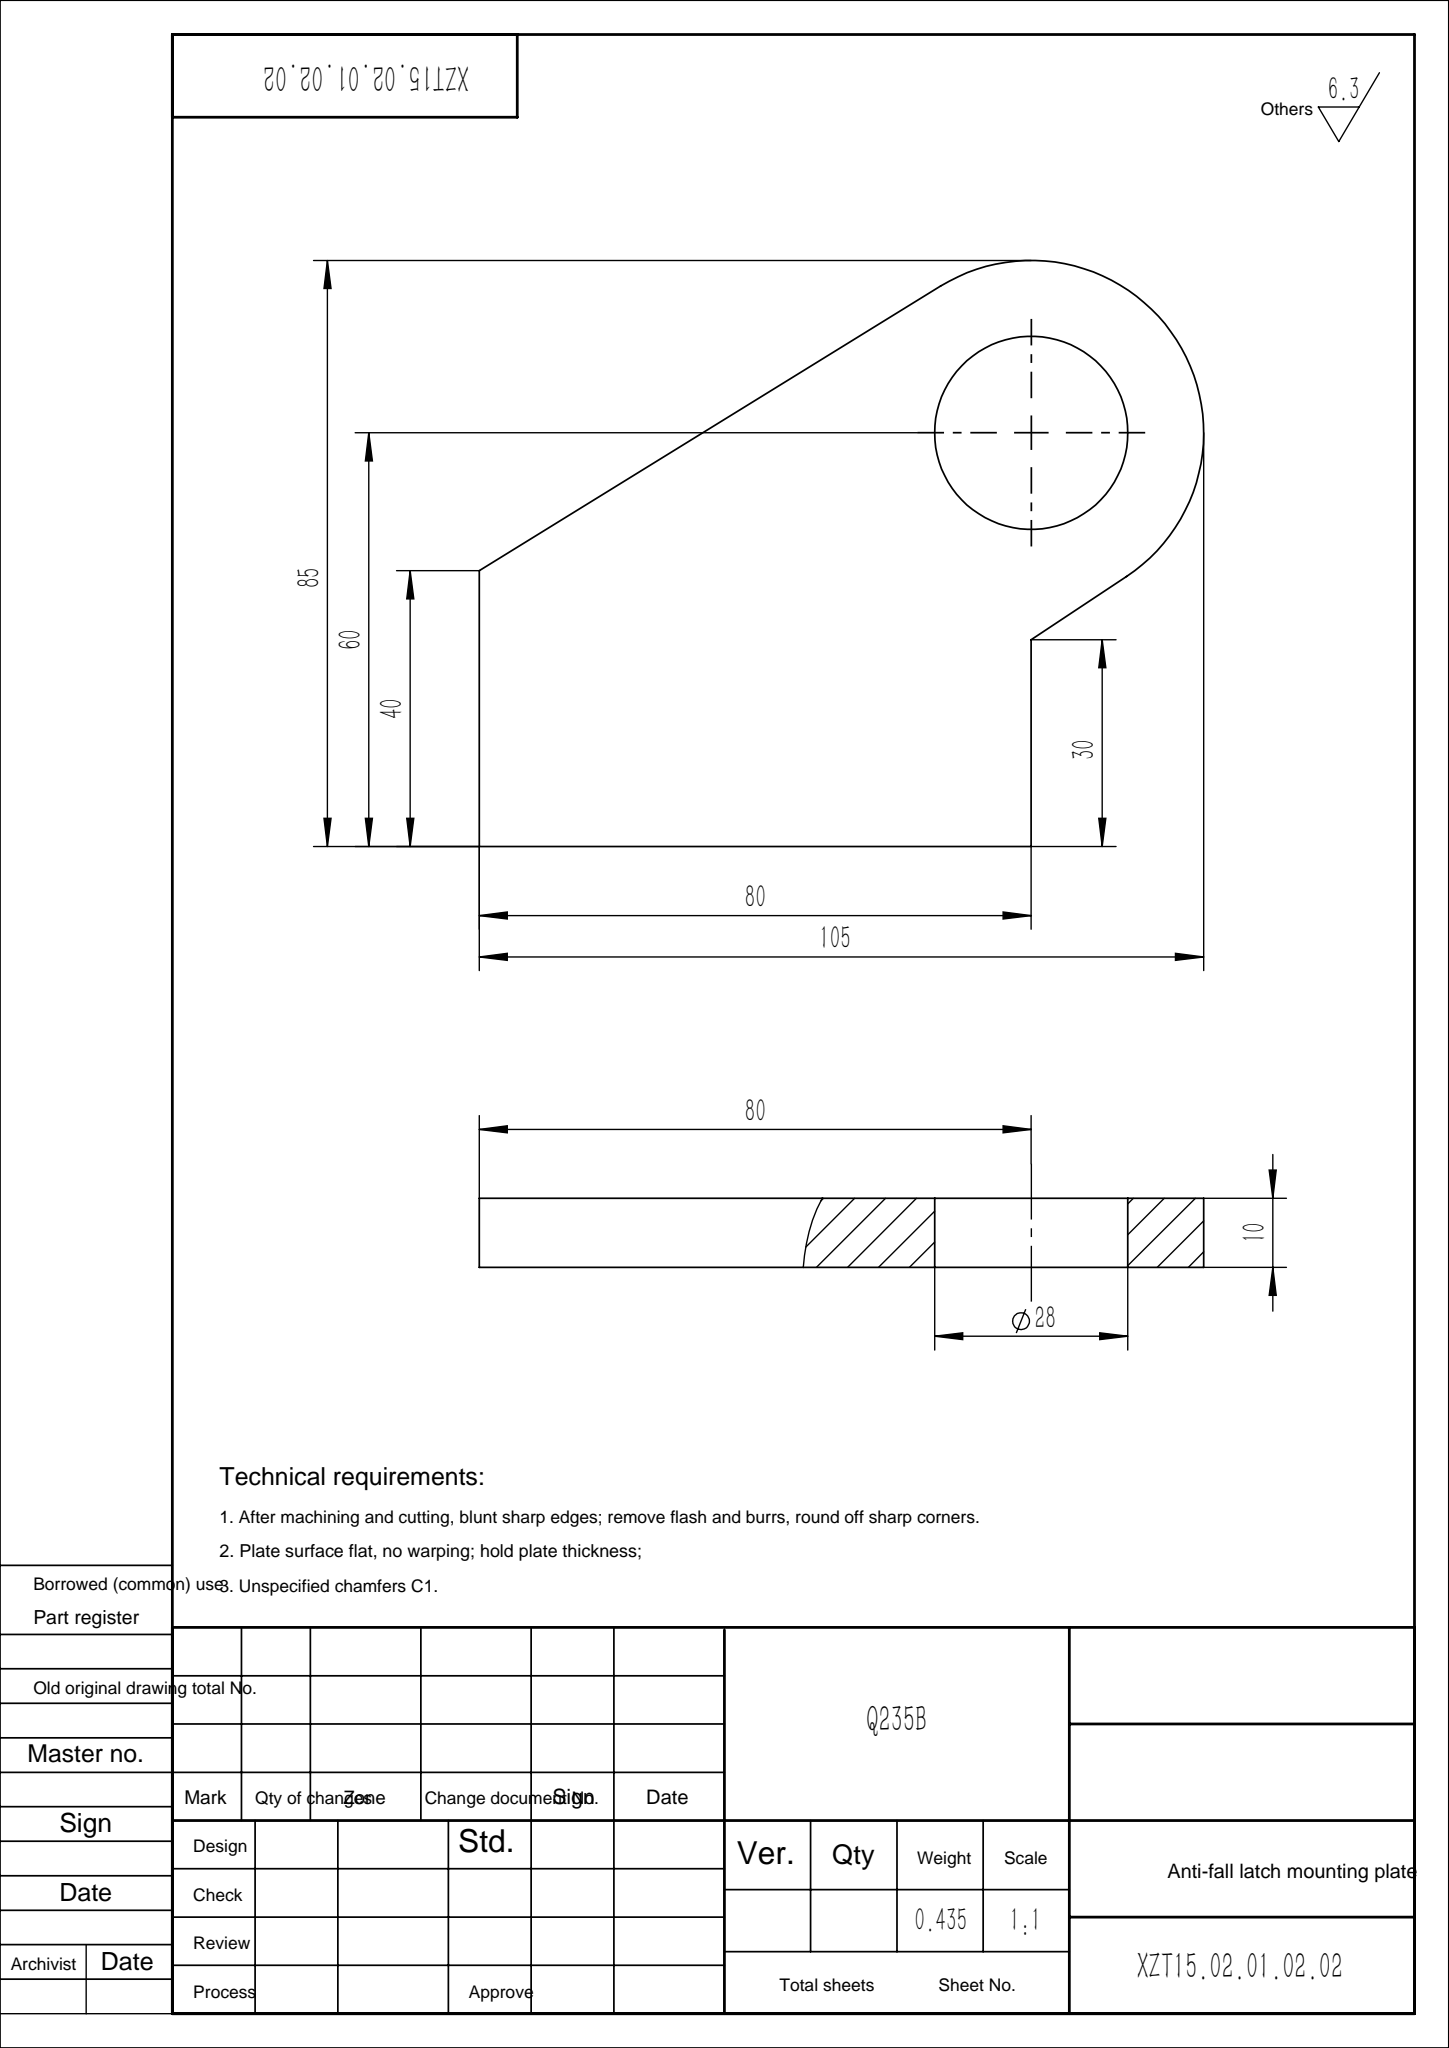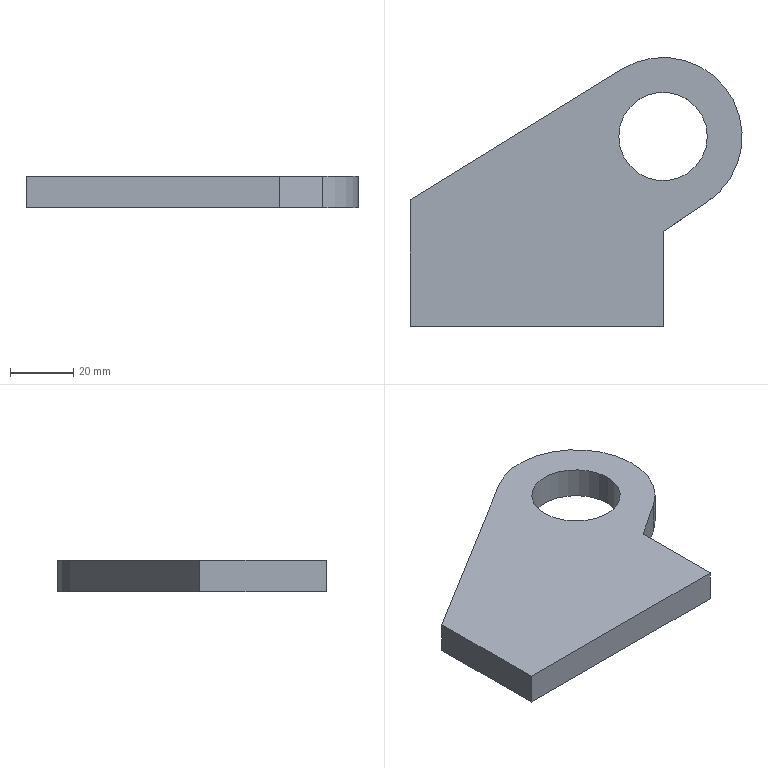Part | SolidWorks | features Extrusion 1 | 1 solid | 10 faces | box 105 x 85 x 10 mm | volume 55453 mm3 | plane 7 | cylinder 3 | commonest cylinder face diameters 28 x2 50 x1
STEP:
#1=CARTESIAN_POINT('',(66.,60.,5.));
#2=VERTEX_POINT('',#1);
#3=CARTESIAN_POINT('',(94.,60.,5.));
#4=VERTEX_POINT('',#3);
#5=CARTESIAN_POINT('',(80.,60.,5.));
#6=DIRECTION('',(0.,0.,1.));
#7=DIRECTION('',(1.,0.,0.));
#8=AXIS2_PLACEMENT_3D('',#5,#6,#7);
#9=CIRCLE('',#8,14.);
#10=EDGE_CURVE('',#2,#4,#9,.T.);
#11=ORIENTED_EDGE('',*,*,#10,.T.);
#12=CARTESIAN_POINT('',(94.,60.,-5.));
#13=VERTEX_POINT('',#12);
#14=CARTESIAN_POINT('',(94.,60.,5.));
#15=DIRECTION('',(0.,0.,-1.));
#16=VECTOR('',#15,1000.);
#17=LINE('',#14,#16);
#18=EDGE_CURVE('',#4,#13,#17,.T.);
#19=ORIENTED_EDGE('',*,*,#18,.T.);
#20=CARTESIAN_POINT('',(66.,60.,-5.));
#21=VERTEX_POINT('',#20);
#22=CARTESIAN_POINT('',(80.,60.,-5.));
#23=DIRECTION('',(0.,0.,1.));
#24=DIRECTION('',(1.,0.,0.));
#25=AXIS2_PLACEMENT_3D('',#22,#23,#24);
#26=CIRCLE('',#25,14.);
#27=EDGE_CURVE('',#21,#13,#26,.T.);
#28=ORIENTED_EDGE('',*,*,#27,.F.);
#29=CARTESIAN_POINT('',(66.,60.,5.));
#30=DIRECTION('',(0.,0.,-1.));
#31=VECTOR('',#30,1000.);
#32=LINE('',#29,#31);
#33=EDGE_CURVE('',#2,#21,#32,.T.);
#34=ORIENTED_EDGE('',*,*,#33,.F.);
#35=EDGE_LOOP('',(#11,#19,#28,#34));
#36=FACE_OUTER_BOUND('',#35,.T.);
#37=CARTESIAN_POINT('',(80.,60.,5.));
#38=DIRECTION('',(0.,0.,-1.));
#39=DIRECTION('',(-1.,0.,0.));
#40=AXIS2_PLACEMENT_3D('',#37,#38,#39);
#41=CYLINDRICAL_SURFACE('',#40,14.);
#42=ADVANCED_FACE('',(#36),#41,.F.);
#43=CARTESIAN_POINT('',(0.,0.,5.));
#44=VERTEX_POINT('',#43);
#45=CARTESIAN_POINT('',(80.,0.,5.));
#46=VERTEX_POINT('',#45);
#47=CARTESIAN_POINT('',(80.,0.,5.));
#48=DIRECTION('',(1.,0.,0.));
#49=VECTOR('',#48,1000.);
#50=LINE('',#47,#49);
#51=EDGE_CURVE('',#44,#46,#50,.T.);
#52=ORIENTED_EDGE('',*,*,#51,.T.);
#53=CARTESIAN_POINT('',(80.,30.,5.));
#54=VERTEX_POINT('',#53);
#55=CARTESIAN_POINT('',(80.,30.,5.));
#56=DIRECTION('',(0.,1.,0.));
#57=VECTOR('',#56,1000.);
#58=LINE('',#55,#57);
#59=EDGE_CURVE('',#46,#54,#58,.T.);
#60=ORIENTED_EDGE('',*,*,#59,.T.);
#61=CARTESIAN_POINT('',(93.819,39.167,5.));
#62=VERTEX_POINT('',#61);
#63=CARTESIAN_POINT('',(80.,30.,5.));
#64=DIRECTION('',(0.8333,0.5528,0.));
#65=VECTOR('',#64,1000.);
#66=LINE('',#63,#65);
#67=EDGE_CURVE('',#54,#62,#66,.T.);
#68=ORIENTED_EDGE('',*,*,#67,.T.);
#69=CARTESIAN_POINT('',(66.869,81.274,5.));
#70=VERTEX_POINT('',#69);
#71=CARTESIAN_POINT('',(80.,60.,5.));
#72=DIRECTION('',(0.,0.,1.));
#73=DIRECTION('',(-1.,0.,0.));
#74=AXIS2_PLACEMENT_3D('',#71,#72,#73);
#75=CIRCLE('',#74,25.);
#76=EDGE_CURVE('',#62,#70,#75,.T.);
#77=ORIENTED_EDGE('',*,*,#76,.T.);
#78=CARTESIAN_POINT('',(0.,40.,5.));
#79=VERTEX_POINT('',#78);
#80=CARTESIAN_POINT('',(0.,40.,5.));
#81=DIRECTION('',(-0.851,-0.5252,0.));
#82=VECTOR('',#81,1000.);
#83=LINE('',#80,#82);
#84=EDGE_CURVE('',#70,#79,#83,.T.);
#85=ORIENTED_EDGE('',*,*,#84,.T.);
#86=CARTESIAN_POINT('',(0.,0.,5.));
#87=DIRECTION('',(0.,-1.,0.));
#88=VECTOR('',#87,1000.);
#89=LINE('',#86,#88);
#90=EDGE_CURVE('',#79,#44,#89,.T.);
#91=ORIENTED_EDGE('',*,*,#90,.T.);
#92=EDGE_LOOP('',(#52,#60,#68,#77,#85,#91));
#93=FACE_OUTER_BOUND('',#92,.T.);
#94=ORIENTED_EDGE('',*,*,#10,.F.);
#95=CARTESIAN_POINT('',(80.,60.,5.));
#96=DIRECTION('',(0.,0.,1.));
#97=DIRECTION('',(1.,0.,0.));
#98=AXIS2_PLACEMENT_3D('',#95,#96,#97);
#99=CIRCLE('',#98,14.);
#100=EDGE_CURVE('',#4,#2,#99,.T.);
#101=ORIENTED_EDGE('',*,*,#100,.F.);
#102=EDGE_LOOP('',(#94,#101));
#103=FACE_BOUND('',#102,.T.);
#104=CARTESIAN_POINT('',(80.,60.,5.));
#105=DIRECTION('',(0.,0.,-1.));
#106=DIRECTION('',(-1.,0.,0.));
#107=AXIS2_PLACEMENT_3D('',#104,#105,#106);
#108=PLANE('',#107);
#109=ADVANCED_FACE('',(#93,#103),#108,.F.);
#110=CARTESIAN_POINT('',(0.,0.,-5.));
#111=VERTEX_POINT('',#110);
#112=CARTESIAN_POINT('',(80.,0.,-5.));
#113=VERTEX_POINT('',#112);
#114=CARTESIAN_POINT('',(80.,0.,-5.));
#115=DIRECTION('',(1.,0.,0.));
#116=VECTOR('',#115,1000.);
#117=LINE('',#114,#116);
#118=EDGE_CURVE('',#111,#113,#117,.T.);
#119=ORIENTED_EDGE('',*,*,#118,.F.);
#120=CARTESIAN_POINT('',(0.,40.,-5.));
#121=VERTEX_POINT('',#120);
#122=CARTESIAN_POINT('',(0.,0.,-5.));
#123=DIRECTION('',(0.,-1.,0.));
#124=VECTOR('',#123,1000.);
#125=LINE('',#122,#124);
#126=EDGE_CURVE('',#121,#111,#125,.T.);
#127=ORIENTED_EDGE('',*,*,#126,.F.);
#128=CARTESIAN_POINT('',(66.869,81.274,-5.));
#129=VERTEX_POINT('',#128);
#130=CARTESIAN_POINT('',(0.,40.,-5.));
#131=DIRECTION('',(-0.851,-0.5252,0.));
#132=VECTOR('',#131,1000.);
#133=LINE('',#130,#132);
#134=EDGE_CURVE('',#129,#121,#133,.T.);
#135=ORIENTED_EDGE('',*,*,#134,.F.);
#136=CARTESIAN_POINT('',(93.819,39.167,-5.));
#137=VERTEX_POINT('',#136);
#138=CARTESIAN_POINT('',(80.,60.,-5.));
#139=DIRECTION('',(0.,0.,1.));
#140=DIRECTION('',(-1.,0.,0.));
#141=AXIS2_PLACEMENT_3D('',#138,#139,#140);
#142=CIRCLE('',#141,25.);
#143=EDGE_CURVE('',#137,#129,#142,.T.);
#144=ORIENTED_EDGE('',*,*,#143,.F.);
#145=CARTESIAN_POINT('',(80.,30.,-5.));
#146=VERTEX_POINT('',#145);
#147=CARTESIAN_POINT('',(80.,30.,-5.));
#148=DIRECTION('',(0.8333,0.5528,0.));
#149=VECTOR('',#148,1000.);
#150=LINE('',#147,#149);
#151=EDGE_CURVE('',#146,#137,#150,.T.);
#152=ORIENTED_EDGE('',*,*,#151,.F.);
#153=CARTESIAN_POINT('',(80.,30.,-5.));
#154=DIRECTION('',(0.,1.,0.));
#155=VECTOR('',#154,1000.);
#156=LINE('',#153,#155);
#157=EDGE_CURVE('',#113,#146,#156,.T.);
#158=ORIENTED_EDGE('',*,*,#157,.F.);
#159=EDGE_LOOP('',(#119,#127,#135,#144,#152,#158));
#160=FACE_OUTER_BOUND('',#159,.T.);
#161=ORIENTED_EDGE('',*,*,#27,.T.);
#162=CARTESIAN_POINT('',(80.,60.,-5.));
#163=DIRECTION('',(0.,0.,1.));
#164=DIRECTION('',(1.,0.,0.));
#165=AXIS2_PLACEMENT_3D('',#162,#163,#164);
#166=CIRCLE('',#165,14.);
#167=EDGE_CURVE('',#13,#21,#166,.T.);
#168=ORIENTED_EDGE('',*,*,#167,.T.);
#169=EDGE_LOOP('',(#161,#168));
#170=FACE_BOUND('',#169,.T.);
#171=CARTESIAN_POINT('',(80.,60.,-5.));
#172=DIRECTION('',(0.,0.,-1.));
#173=DIRECTION('',(-1.,0.,0.));
#174=AXIS2_PLACEMENT_3D('',#171,#172,#173);
#175=PLANE('',#174);
#176=ADVANCED_FACE('',(#160,#170),#175,.T.);
#177=ORIENTED_EDGE('',*,*,#118,.T.);
#178=CARTESIAN_POINT('',(80.,0.,5.));
#179=DIRECTION('',(0.,0.,-1.));
#180=VECTOR('',#179,1000.);
#181=LINE('',#178,#180);
#182=EDGE_CURVE('',#46,#113,#181,.T.);
#183=ORIENTED_EDGE('',*,*,#182,.F.);
#184=ORIENTED_EDGE('',*,*,#51,.F.);
#185=CARTESIAN_POINT('',(0.,0.,5.));
#186=DIRECTION('',(0.,0.,-1.));
#187=VECTOR('',#186,1000.);
#188=LINE('',#185,#187);
#189=EDGE_CURVE('',#44,#111,#188,.T.);
#190=ORIENTED_EDGE('',*,*,#189,.T.);
#191=EDGE_LOOP('',(#177,#183,#184,#190));
#192=FACE_OUTER_BOUND('',#191,.T.);
#193=CARTESIAN_POINT('',(80.,0.,5.));
#194=DIRECTION('',(0.,1.,0.));
#195=DIRECTION('',(0.,0.,1.));
#196=AXIS2_PLACEMENT_3D('',#193,#194,#195);
#197=PLANE('',#196);
#198=ADVANCED_FACE('',(#192),#197,.F.);
#199=ORIENTED_EDGE('',*,*,#157,.T.);
#200=CARTESIAN_POINT('',(80.,30.,5.));
#201=DIRECTION('',(0.,0.,-1.));
#202=VECTOR('',#201,1000.);
#203=LINE('',#200,#202);
#204=EDGE_CURVE('',#54,#146,#203,.T.);
#205=ORIENTED_EDGE('',*,*,#204,.F.);
#206=ORIENTED_EDGE('',*,*,#59,.F.);
#207=ORIENTED_EDGE('',*,*,#182,.T.);
#208=EDGE_LOOP('',(#199,#205,#206,#207));
#209=FACE_OUTER_BOUND('',#208,.T.);
#210=CARTESIAN_POINT('',(80.,30.,5.));
#211=DIRECTION('',(-1.,0.,0.));
#212=DIRECTION('',(0.,0.,1.));
#213=AXIS2_PLACEMENT_3D('',#210,#211,#212);
#214=PLANE('',#213);
#215=ADVANCED_FACE('',(#209),#214,.F.);
#216=ORIENTED_EDGE('',*,*,#151,.T.);
#217=CARTESIAN_POINT('',(93.819,39.167,5.));
#218=DIRECTION('',(0.,0.,-1.));
#219=VECTOR('',#218,1000.);
#220=LINE('',#217,#219);
#221=EDGE_CURVE('',#62,#137,#220,.T.);
#222=ORIENTED_EDGE('',*,*,#221,.F.);
#223=ORIENTED_EDGE('',*,*,#67,.F.);
#224=ORIENTED_EDGE('',*,*,#204,.T.);
#225=EDGE_LOOP('',(#216,#222,#223,#224));
#226=FACE_OUTER_BOUND('',#225,.T.);
#227=CARTESIAN_POINT('',(80.,30.,5.));
#228=DIRECTION('',(-0.5528,0.8333,0.));
#229=DIRECTION('',(-0.8333,-0.5528,0.));
#230=AXIS2_PLACEMENT_3D('',#227,#228,#229);
#231=PLANE('',#230);
#232=ADVANCED_FACE('',(#226),#231,.F.);
#233=ORIENTED_EDGE('',*,*,#143,.T.);
#234=CARTESIAN_POINT('',(66.869,81.274,5.));
#235=DIRECTION('',(0.,0.,-1.));
#236=VECTOR('',#235,1000.);
#237=LINE('',#234,#236);
#238=EDGE_CURVE('',#70,#129,#237,.T.);
#239=ORIENTED_EDGE('',*,*,#238,.F.);
#240=ORIENTED_EDGE('',*,*,#76,.F.);
#241=ORIENTED_EDGE('',*,*,#221,.T.);
#242=EDGE_LOOP('',(#233,#239,#240,#241));
#243=FACE_OUTER_BOUND('',#242,.T.);
#244=CARTESIAN_POINT('',(80.,60.,5.));
#245=DIRECTION('',(0.,0.,-1.));
#246=DIRECTION('',(-1.,0.,0.));
#247=AXIS2_PLACEMENT_3D('',#244,#245,#246);
#248=CYLINDRICAL_SURFACE('',#247,25.);
#249=ADVANCED_FACE('',(#243),#248,.T.);
#250=ORIENTED_EDGE('',*,*,#134,.T.);
#251=CARTESIAN_POINT('',(0.,40.,5.));
#252=DIRECTION('',(0.,0.,-1.));
#253=VECTOR('',#252,1000.);
#254=LINE('',#251,#253);
#255=EDGE_CURVE('',#79,#121,#254,.T.);
#256=ORIENTED_EDGE('',*,*,#255,.F.);
#257=ORIENTED_EDGE('',*,*,#84,.F.);
#258=ORIENTED_EDGE('',*,*,#238,.T.);
#259=EDGE_LOOP('',(#250,#256,#257,#258));
#260=FACE_OUTER_BOUND('',#259,.T.);
#261=CARTESIAN_POINT('',(0.,40.,5.));
#262=DIRECTION('',(0.5252,-0.851,0.));
#263=DIRECTION('',(0.851,0.5252,0.));
#264=AXIS2_PLACEMENT_3D('',#261,#262,#263);
#265=PLANE('',#264);
#266=ADVANCED_FACE('',(#260),#265,.F.);
#267=ORIENTED_EDGE('',*,*,#126,.T.);
#268=ORIENTED_EDGE('',*,*,#189,.F.);
#269=ORIENTED_EDGE('',*,*,#90,.F.);
#270=ORIENTED_EDGE('',*,*,#255,.T.);
#271=EDGE_LOOP('',(#267,#268,#269,#270));
#272=FACE_OUTER_BOUND('',#271,.T.);
#273=CARTESIAN_POINT('',(0.,0.,5.));
#274=DIRECTION('',(1.,0.,0.));
#275=DIRECTION('',(0.,0.,-1.));
#276=AXIS2_PLACEMENT_3D('',#273,#274,#275);
#277=PLANE('',#276);
#278=ADVANCED_FACE('',(#272),#277,.F.);
#279=ORIENTED_EDGE('',*,*,#18,.F.);
#280=ORIENTED_EDGE('',*,*,#100,.T.);
#281=ORIENTED_EDGE('',*,*,#33,.T.);
#282=ORIENTED_EDGE('',*,*,#167,.F.);
#283=EDGE_LOOP('',(#279,#280,#281,#282));
#284=FACE_OUTER_BOUND('',#283,.T.);
#285=CARTESIAN_POINT('',(80.,60.,5.));
#286=DIRECTION('',(0.,0.,-1.));
#287=DIRECTION('',(-1.,0.,0.));
#288=AXIS2_PLACEMENT_3D('',#285,#286,#287);
#289=CYLINDRICAL_SURFACE('',#288,14.);
#290=ADVANCED_FACE('',(#284),#289,.F.);
#291=CLOSED_SHELL('',(#42,#109,#176,#198,#215,#232,#249,#266,#278,#290));
#292=MANIFOLD_SOLID_BREP('',#291);
#293=CARTESIAN_POINT('',(0.,0.,0.));
#294=DIRECTION('',(0.,0.,1.));
#295=DIRECTION('',(1.,0.,0.));
#296=AXIS2_PLACEMENT_3D('',#293,#294,#295);
#297=(LENGTH_UNIT()NAMED_UNIT(*)SI_UNIT(.MILLI.,.METRE.));
#298=UNCERTAINTY_MEASURE_WITH_UNIT(LENGTH_MEASURE(0.00001),#297,'','');
#299=(NAMED_UNIT(*)PLANE_ANGLE_UNIT()SI_UNIT($,.RADIAN.));
#300=(NAMED_UNIT(*)SI_UNIT($,.STERADIAN.)SOLID_ANGLE_UNIT());
#301=(GEOMETRIC_REPRESENTATION_CONTEXT(3)GLOBAL_UNCERTAINTY_ASSIGNED_CONTEXT((#298))GLOBAL_UNIT_ASSIGNED_CONTEXT((#297,#299,#300))REPRESENTATION_CONTEXT('',''));
#302=ADVANCED_BREP_SHAPE_REPRESENTATION('',(#292,#296),#301);